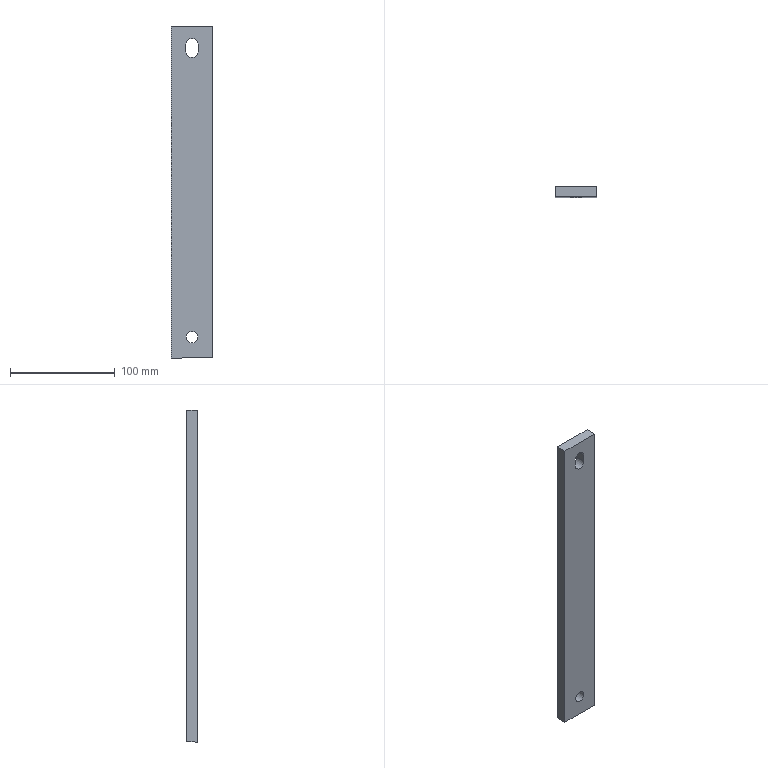Part | STEP file | 1 solid | 11 faces | box 40 x 10 x 317 mm | volume 124006 mm3 | plane 8 | cylinder 3 | commonest cylinder face diameters 11.5 x2 11 x1
STEP:
#1=CARTESIAN_POINT('',(260.75,302.5,202.5));
#2=VERTEX_POINT('',#1);
#3=CARTESIAN_POINT('',(260.75,302.5,195.5));
#4=VERTEX_POINT('',#3);
#5=CARTESIAN_POINT('',(260.75,302.5,52.));
#6=DIRECTION('',(0.,0.,-1.));
#7=VECTOR('',#6,1.);
#8=LINE('',#5,#7);
#9=EDGE_CURVE('',#2,#4,#8,.T.);
#10=ORIENTED_EDGE('',*,*,#9,.F.);
#11=CARTESIAN_POINT('',(249.25,302.5,202.5));
#12=VERTEX_POINT('',#11);
#13=CARTESIAN_POINT('',(255.,302.5,202.5));
#14=DIRECTION('',(0.,1.,0.));
#15=DIRECTION('',(0.,0.,1.));
#16=AXIS2_PLACEMENT_3D('',#13,#14,#15);
#17=CIRCLE('',#16,5.75);
#18=EDGE_CURVE('',#12,#2,#17,.T.);
#19=ORIENTED_EDGE('',*,*,#18,.F.);
#20=CARTESIAN_POINT('',(249.25,302.5,195.5));
#21=VERTEX_POINT('',#20);
#22=CARTESIAN_POINT('',(249.25,302.5,52.));
#23=DIRECTION('',(0.,0.,-1.));
#24=VECTOR('',#23,1.);
#25=LINE('',#22,#24);
#26=EDGE_CURVE('',#12,#21,#25,.T.);
#27=ORIENTED_EDGE('',*,*,#26,.T.);
#28=CARTESIAN_POINT('',(255.,302.5,195.5));
#29=DIRECTION('',(0.,1.,0.));
#30=DIRECTION('',(0.,0.,1.));
#31=AXIS2_PLACEMENT_3D('',#28,#29,#30);
#32=CIRCLE('',#31,5.75);
#33=EDGE_CURVE('',#4,#21,#32,.T.);
#34=ORIENTED_EDGE('',*,*,#33,.F.);
#35=EDGE_LOOP('',(#10,#19,#27,#34));
#36=FACE_BOUND('',#35,.T.);
#37=CARTESIAN_POINT('',(235.,302.5,-97.));
#38=VERTEX_POINT('',#37);
#39=CARTESIAN_POINT('',(275.,302.5,-97.));
#40=VERTEX_POINT('',#39);
#41=CARTESIAN_POINT('',(118.5,302.5,-97.));
#42=DIRECTION('',(1.,0.,0.));
#43=VECTOR('',#42,1.);
#44=LINE('',#41,#43);
#45=EDGE_CURVE('',#38,#40,#44,.T.);
#46=ORIENTED_EDGE('',*,*,#45,.F.);
#47=CARTESIAN_POINT('',(235.,302.5,220.));
#48=VERTEX_POINT('',#47);
#49=CARTESIAN_POINT('',(235.,302.5,155.));
#50=DIRECTION('',(0.,0.,1.));
#51=VECTOR('',#50,1.);
#52=LINE('',#49,#51);
#53=EDGE_CURVE('',#38,#48,#52,.T.);
#54=ORIENTED_EDGE('',*,*,#53,.T.);
#55=CARTESIAN_POINT('',(275.,302.5,220.));
#56=VERTEX_POINT('',#55);
#57=CARTESIAN_POINT('',(131.,302.5,220.));
#58=DIRECTION('',(1.,0.,0.));
#59=VECTOR('',#58,1.);
#60=LINE('',#57,#59);
#61=EDGE_CURVE('',#48,#56,#60,.T.);
#62=ORIENTED_EDGE('',*,*,#61,.T.);
#63=CARTESIAN_POINT('',(275.,302.5,155.));
#64=DIRECTION('',(0.,0.,1.));
#65=VECTOR('',#64,1.);
#66=LINE('',#63,#65);
#67=EDGE_CURVE('',#40,#56,#66,.T.);
#68=ORIENTED_EDGE('',*,*,#67,.F.);
#69=EDGE_LOOP('',(#46,#54,#62,#68));
#70=FACE_BOUND('',#69,.T.);
#71=CARTESIAN_POINT('',(249.5,302.5,-77.));
#72=VERTEX_POINT('',#71);
#73=CARTESIAN_POINT('',(255.,302.5,-77.));
#74=DIRECTION('',(0.,1.,0.));
#75=DIRECTION('',(-1.,0.,0.));
#76=AXIS2_PLACEMENT_3D('',#73,#74,#75);
#77=CIRCLE('',#76,5.5);
#78=EDGE_CURVE('',#72,#72,#77,.T.);
#79=ORIENTED_EDGE('',*,*,#78,.F.);
#80=EDGE_LOOP('',(#79));
#81=FACE_BOUND('',#80,.T.);
#82=CARTESIAN_POINT('',(131.,302.5,-22.));
#83=DIRECTION('',(0.,1.,0.));
#84=DIRECTION('',(0.,0.,-1.));
#85=AXIS2_PLACEMENT_3D('',#82,#83,#84);
#86=PLANE('',#85);
#87=ADVANCED_FACE('',(#36,#70,#81),#86,.T.);
#88=CARTESIAN_POINT('',(235.,292.5,-97.));
#89=VERTEX_POINT('',#88);
#90=CARTESIAN_POINT('',(235.,-1.,-97.));
#91=DIRECTION('',(0.,-1.,0.));
#92=VECTOR('',#91,1.);
#93=LINE('',#90,#92);
#94=EDGE_CURVE('',#38,#89,#93,.T.);
#95=ORIENTED_EDGE('',*,*,#94,.T.);
#96=CARTESIAN_POINT('',(235.,292.5,220.));
#97=VERTEX_POINT('',#96);
#98=CARTESIAN_POINT('',(235.,292.5,130.));
#99=DIRECTION('',(0.,0.,-1.));
#100=VECTOR('',#99,1.);
#101=LINE('',#98,#100);
#102=EDGE_CURVE('',#97,#89,#101,.T.);
#103=ORIENTED_EDGE('',*,*,#102,.F.);
#104=CARTESIAN_POINT('',(235.,-7.4,220.));
#105=DIRECTION('',(0.,-1.,0.));
#106=VECTOR('',#105,1.);
#107=LINE('',#104,#106);
#108=EDGE_CURVE('',#48,#97,#107,.T.);
#109=ORIENTED_EDGE('',*,*,#108,.F.);
#110=ORIENTED_EDGE('',*,*,#53,.F.);
#111=EDGE_LOOP('',(#95,#103,#109,#110));
#112=FACE_OUTER_BOUND('',#111,.T.);
#113=CARTESIAN_POINT('',(235.,-7.4,155.));
#114=DIRECTION('',(-1.,0.,0.));
#115=DIRECTION('',(0.,-1.,0.));
#116=AXIS2_PLACEMENT_3D('',#113,#114,#115);
#117=PLANE('',#116);
#118=ADVANCED_FACE('',(#112),#117,.T.);
#119=CARTESIAN_POINT('',(275.,292.5,-97.));
#120=VERTEX_POINT('',#119);
#121=CARTESIAN_POINT('',(275.,292.5,220.));
#122=VERTEX_POINT('',#121);
#123=CARTESIAN_POINT('',(275.,292.5,155.));
#124=DIRECTION('',(0.,0.,1.));
#125=VECTOR('',#124,1.);
#126=LINE('',#123,#125);
#127=EDGE_CURVE('',#120,#122,#126,.T.);
#128=ORIENTED_EDGE('',*,*,#127,.F.);
#129=CARTESIAN_POINT('',(275.,-1.,-97.));
#130=DIRECTION('',(0.,-1.,0.));
#131=VECTOR('',#130,1.);
#132=LINE('',#129,#131);
#133=EDGE_CURVE('',#40,#120,#132,.T.);
#134=ORIENTED_EDGE('',*,*,#133,.F.);
#135=ORIENTED_EDGE('',*,*,#67,.T.);
#136=CARTESIAN_POINT('',(275.,-7.4,220.));
#137=DIRECTION('',(0.,-1.,0.));
#138=VECTOR('',#137,1.);
#139=LINE('',#136,#138);
#140=EDGE_CURVE('',#56,#122,#139,.T.);
#141=ORIENTED_EDGE('',*,*,#140,.T.);
#142=EDGE_LOOP('',(#128,#134,#135,#141));
#143=FACE_OUTER_BOUND('',#142,.T.);
#144=CARTESIAN_POINT('',(275.,-7.4,155.));
#145=DIRECTION('',(-1.,0.,0.));
#146=DIRECTION('',(0.,-1.,0.));
#147=AXIS2_PLACEMENT_3D('',#144,#145,#146);
#148=PLANE('',#147);
#149=ADVANCED_FACE('',(#143),#148,.F.);
#150=CARTESIAN_POINT('',(88.5,292.5,220.));
#151=DIRECTION('',(-1.,0.,0.));
#152=VECTOR('',#151,1.);
#153=LINE('',#150,#152);
#154=EDGE_CURVE('',#122,#97,#153,.T.);
#155=ORIENTED_EDGE('',*,*,#154,.F.);
#156=ORIENTED_EDGE('',*,*,#140,.F.);
#157=ORIENTED_EDGE('',*,*,#61,.F.);
#158=ORIENTED_EDGE('',*,*,#108,.T.);
#159=EDGE_LOOP('',(#155,#156,#157,#158));
#160=FACE_OUTER_BOUND('',#159,.T.);
#161=CARTESIAN_POINT('',(88.5,-1.,220.));
#162=DIRECTION('',(0.,0.,-1.));
#163=DIRECTION('',(1.,0.,0.));
#164=AXIS2_PLACEMENT_3D('',#161,#162,#163);
#165=PLANE('',#164);
#166=ADVANCED_FACE('',(#160),#165,.F.);
#167=CARTESIAN_POINT('',(118.5,292.5,-97.));
#168=DIRECTION('',(1.,0.,0.));
#169=VECTOR('',#168,1.);
#170=LINE('',#167,#169);
#171=EDGE_CURVE('',#89,#120,#170,.T.);
#172=ORIENTED_EDGE('',*,*,#171,.F.);
#173=ORIENTED_EDGE('',*,*,#94,.F.);
#174=ORIENTED_EDGE('',*,*,#45,.T.);
#175=ORIENTED_EDGE('',*,*,#133,.T.);
#176=EDGE_LOOP('',(#172,#173,#174,#175));
#177=FACE_OUTER_BOUND('',#176,.T.);
#178=CARTESIAN_POINT('',(118.5,-1.,-97.));
#179=DIRECTION('',(0.,0.,1.));
#180=DIRECTION('',(1.,0.,0.));
#181=AXIS2_PLACEMENT_3D('',#178,#179,#180);
#182=PLANE('',#181);
#183=ADVANCED_FACE('',(#177),#182,.F.);
#184=CARTESIAN_POINT('',(260.5,292.5,-77.));
#185=VERTEX_POINT('',#184);
#186=CARTESIAN_POINT('',(255.,292.5,-77.));
#187=DIRECTION('',(0.,1.,0.));
#188=DIRECTION('',(1.,0.,0.));
#189=AXIS2_PLACEMENT_3D('',#186,#187,#188);
#190=CIRCLE('',#189,5.5);
#191=EDGE_CURVE('',#185,#185,#190,.T.);
#192=ORIENTED_EDGE('',*,*,#191,.T.);
#193=EDGE_LOOP('',(#192));
#194=FACE_BOUND('',#193,.T.);
#195=CARTESIAN_POINT('',(249.25,292.5,202.5));
#196=VERTEX_POINT('',#195);
#197=CARTESIAN_POINT('',(260.75,292.5,202.5));
#198=VERTEX_POINT('',#197);
#199=CARTESIAN_POINT('',(255.,292.5,202.5));
#200=DIRECTION('',(0.,1.,0.));
#201=DIRECTION('',(0.,0.,1.));
#202=AXIS2_PLACEMENT_3D('',#199,#200,#201);
#203=CIRCLE('',#202,5.75);
#204=EDGE_CURVE('',#196,#198,#203,.T.);
#205=ORIENTED_EDGE('',*,*,#204,.T.);
#206=CARTESIAN_POINT('',(260.75,292.5,195.5));
#207=VERTEX_POINT('',#206);
#208=CARTESIAN_POINT('',(260.75,292.5,204.));
#209=DIRECTION('',(0.,0.,-1.));
#210=VECTOR('',#209,1.);
#211=LINE('',#208,#210);
#212=EDGE_CURVE('',#198,#207,#211,.T.);
#213=ORIENTED_EDGE('',*,*,#212,.T.);
#214=CARTESIAN_POINT('',(249.25,292.5,195.5));
#215=VERTEX_POINT('',#214);
#216=CARTESIAN_POINT('',(255.,292.5,195.5));
#217=DIRECTION('',(0.,1.,0.));
#218=DIRECTION('',(0.,0.,1.));
#219=AXIS2_PLACEMENT_3D('',#216,#217,#218);
#220=CIRCLE('',#219,5.75);
#221=EDGE_CURVE('',#207,#215,#220,.T.);
#222=ORIENTED_EDGE('',*,*,#221,.T.);
#223=CARTESIAN_POINT('',(249.25,292.5,204.));
#224=DIRECTION('',(0.,0.,-1.));
#225=VECTOR('',#224,1.);
#226=LINE('',#223,#225);
#227=EDGE_CURVE('',#196,#215,#226,.T.);
#228=ORIENTED_EDGE('',*,*,#227,.F.);
#229=EDGE_LOOP('',(#205,#213,#222,#228));
#230=FACE_BOUND('',#229,.T.);
#231=ORIENTED_EDGE('',*,*,#127,.T.);
#232=ORIENTED_EDGE('',*,*,#154,.T.);
#233=ORIENTED_EDGE('',*,*,#102,.T.);
#234=ORIENTED_EDGE('',*,*,#171,.T.);
#235=EDGE_LOOP('',(#231,#232,#233,#234));
#236=FACE_BOUND('',#235,.T.);
#237=CARTESIAN_POINT('',(25.,292.5,130.));
#238=DIRECTION('',(0.,1.,0.));
#239=DIRECTION('',(0.,0.,1.));
#240=AXIS2_PLACEMENT_3D('',#237,#238,#239);
#241=PLANE('',#240);
#242=ADVANCED_FACE('',(#194,#230,#236),#241,.F.);
#243=ORIENTED_EDGE('',*,*,#9,.T.);
#244=CARTESIAN_POINT('',(260.75,291.5,195.5));
#245=DIRECTION('',(0.,-1.,0.));
#246=VECTOR('',#245,1.);
#247=LINE('',#244,#246);
#248=EDGE_CURVE('',#4,#207,#247,.T.);
#249=ORIENTED_EDGE('',*,*,#248,.T.);
#250=ORIENTED_EDGE('',*,*,#212,.F.);
#251=CARTESIAN_POINT('',(260.75,291.5,202.5));
#252=DIRECTION('',(0.,-1.,0.));
#253=VECTOR('',#252,1.);
#254=LINE('',#251,#253);
#255=EDGE_CURVE('',#2,#198,#254,.T.);
#256=ORIENTED_EDGE('',*,*,#255,.F.);
#257=EDGE_LOOP('',(#243,#249,#250,#256));
#258=FACE_OUTER_BOUND('',#257,.T.);
#259=CARTESIAN_POINT('',(260.75,291.5,137.5));
#260=DIRECTION('',(1.,0.,0.));
#261=DIRECTION('',(0.,0.,-1.));
#262=AXIS2_PLACEMENT_3D('',#259,#260,#261);
#263=PLANE('',#262);
#264=ADVANCED_FACE('',(#258),#263,.F.);
#265=ORIENTED_EDGE('',*,*,#33,.T.);
#266=CARTESIAN_POINT('',(249.25,291.5,195.5));
#267=DIRECTION('',(0.,-1.,0.));
#268=VECTOR('',#267,1.);
#269=LINE('',#266,#268);
#270=EDGE_CURVE('',#21,#215,#269,.T.);
#271=ORIENTED_EDGE('',*,*,#270,.T.);
#272=ORIENTED_EDGE('',*,*,#221,.F.);
#273=ORIENTED_EDGE('',*,*,#248,.F.);
#274=EDGE_LOOP('',(#265,#271,#272,#273));
#275=FACE_OUTER_BOUND('',#274,.T.);
#276=CARTESIAN_POINT('',(255.,291.5,195.5));
#277=DIRECTION('',(0.,1.,0.));
#278=DIRECTION('',(0.,0.,1.));
#279=AXIS2_PLACEMENT_3D('',#276,#277,#278);
#280=CYLINDRICAL_SURFACE('',#279,5.75);
#281=ADVANCED_FACE('',(#275),#280,.F.);
#282=CARTESIAN_POINT('',(249.25,291.5,202.5));
#283=DIRECTION('',(0.,-1.,0.));
#284=VECTOR('',#283,1.);
#285=LINE('',#282,#284);
#286=EDGE_CURVE('',#12,#196,#285,.T.);
#287=ORIENTED_EDGE('',*,*,#286,.T.);
#288=ORIENTED_EDGE('',*,*,#227,.T.);
#289=ORIENTED_EDGE('',*,*,#270,.F.);
#290=ORIENTED_EDGE('',*,*,#26,.F.);
#291=EDGE_LOOP('',(#287,#288,#289,#290));
#292=FACE_OUTER_BOUND('',#291,.T.);
#293=CARTESIAN_POINT('',(249.25,291.5,137.5));
#294=DIRECTION('',(1.,0.,0.));
#295=DIRECTION('',(0.,0.,-1.));
#296=AXIS2_PLACEMENT_3D('',#293,#294,#295);
#297=PLANE('',#296);
#298=ADVANCED_FACE('',(#292),#297,.T.);
#299=ORIENTED_EDGE('',*,*,#18,.T.);
#300=ORIENTED_EDGE('',*,*,#255,.T.);
#301=ORIENTED_EDGE('',*,*,#204,.F.);
#302=ORIENTED_EDGE('',*,*,#286,.F.);
#303=EDGE_LOOP('',(#299,#300,#301,#302));
#304=FACE_OUTER_BOUND('',#303,.T.);
#305=CARTESIAN_POINT('',(255.,291.5,202.5));
#306=DIRECTION('',(0.,1.,0.));
#307=DIRECTION('',(0.,0.,1.));
#308=AXIS2_PLACEMENT_3D('',#305,#306,#307);
#309=CYLINDRICAL_SURFACE('',#308,5.75);
#310=ADVANCED_FACE('',(#304),#309,.F.);
#311=ORIENTED_EDGE('',*,*,#78,.T.);
#312=EDGE_LOOP('',(#311));
#313=FACE_BOUND('',#312,.T.);
#314=ORIENTED_EDGE('',*,*,#191,.F.);
#315=EDGE_LOOP('',(#314));
#316=FACE_BOUND('',#315,.T.);
#317=CARTESIAN_POINT('',(255.,292.5,-77.));
#318=DIRECTION('',(0.,1.,0.));
#319=DIRECTION('',(1.,0.,0.));
#320=AXIS2_PLACEMENT_3D('',#317,#318,#319);
#321=CYLINDRICAL_SURFACE('',#320,5.5);
#322=ADVANCED_FACE('',(#313,#316),#321,.F.);
#323=CLOSED_SHELL('',(#87,#118,#149,#166,#183,#242,#264,#281,#298,#310,#322));
#324=MANIFOLD_SOLID_BREP('',#323);
#325=(LENGTH_UNIT()NAMED_UNIT(*)SI_UNIT(.MILLI.,.METRE.));
#326=UNCERTAINTY_MEASURE_WITH_UNIT(LENGTH_MEASURE(0.00002),#325,'','');
#327=(NAMED_UNIT(*)PLANE_ANGLE_UNIT()SI_UNIT($,.RADIAN.));
#328=PLANE_ANGLE_MEASURE_WITH_UNIT(PLANE_ANGLE_MEASURE(0.01745),#327);
#329=DIMENSIONAL_EXPONENTS(0.,0.,0.,0.,0.,0.,0.);
#330=(CONVERSION_BASED_UNIT('DEGREE',#328)NAMED_UNIT(#329)PLANE_ANGLE_UNIT());
#331=(NAMED_UNIT(*)SI_UNIT($,.STERADIAN.)SOLID_ANGLE_UNIT());
#332=(GEOMETRIC_REPRESENTATION_CONTEXT(3)GLOBAL_UNCERTAINTY_ASSIGNED_CONTEXT((#326))GLOBAL_UNIT_ASSIGNED_CONTEXT((#325,#330,#331))REPRESENTATION_CONTEXT('',''));
#333=ADVANCED_BREP_SHAPE_REPRESENTATION('',(#324),#332);